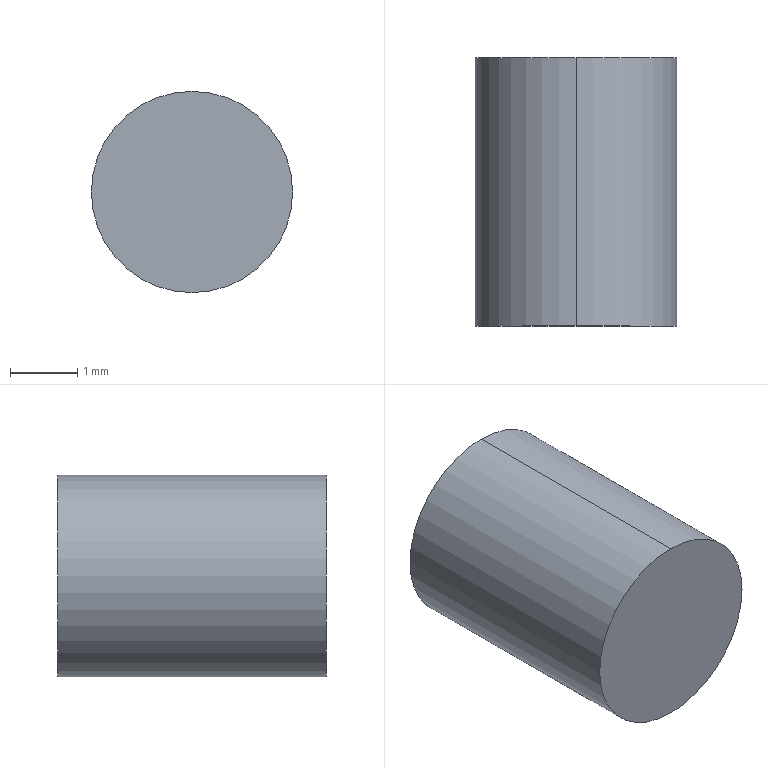Part | NX | features solid 2 | 1 solid | 4 faces | box 3 x 4 x 3 mm | volume 28.274 mm3 | plane 2 | cylinder 2 | commonest cylinder face diameters 3 x2
STEP:
#1=CARTESIAN_POINT('',(250.,-4.,-919.17));
#2=VERTEX_POINT('',#1);
#3=CARTESIAN_POINT('',(250.,-4.,-922.17));
#4=VERTEX_POINT('',#3);
#5=CARTESIAN_POINT('',(250.,-4.,-920.67));
#6=DIRECTION('',(0.,1.,0.));
#7=DIRECTION('',(0.,0.,1.));
#8=AXIS2_PLACEMENT_3D('',#5,#6,#7);
#9=CIRCLE('',#8,1.5);
#10=EDGE_CURVE('',#2,#4,#9,.T.);
#11=ORIENTED_EDGE('',*,*,#10,.F.);
#12=CARTESIAN_POINT('',(250.,-4.,-920.67));
#13=DIRECTION('',(0.,1.,0.));
#14=DIRECTION('',(0.,0.,-1.));
#15=AXIS2_PLACEMENT_3D('',#12,#13,#14);
#16=CIRCLE('',#15,1.5);
#17=EDGE_CURVE('',#4,#2,#16,.T.);
#18=ORIENTED_EDGE('',*,*,#17,.F.);
#19=EDGE_LOOP('',(#11,#18));
#20=FACE_BOUND('',#19,.T.);
#21=CARTESIAN_POINT('',(250.,-4.,-920.67));
#22=DIRECTION('',(0.,1.,0.));
#23=DIRECTION('',(0.,0.,1.));
#24=AXIS2_PLACEMENT_3D('',#21,#22,#23);
#25=PLANE('',#24);
#26=ADVANCED_FACE('',(#20),#25,.F.);
#27=CARTESIAN_POINT('',(250.,0.,-919.17));
#28=VERTEX_POINT('',#27);
#29=CARTESIAN_POINT('',(250.,-4.,-919.17));
#30=DIRECTION('',(0.,1.,0.));
#31=VECTOR('',#30,1000.);
#32=LINE('',#29,#31);
#33=EDGE_CURVE('',#2,#28,#32,.T.);
#34=ORIENTED_EDGE('',*,*,#33,.T.);
#35=CARTESIAN_POINT('',(250.,0.,-922.17));
#36=VERTEX_POINT('',#35);
#37=CARTESIAN_POINT('',(250.,0.,-920.67));
#38=DIRECTION('',(0.,-1.,0.));
#39=DIRECTION('',(0.,0.,1.));
#40=AXIS2_PLACEMENT_3D('',#37,#38,#39);
#41=CIRCLE('',#40,1.5);
#42=EDGE_CURVE('',#28,#36,#41,.T.);
#43=ORIENTED_EDGE('',*,*,#42,.T.);
#44=CARTESIAN_POINT('',(250.,-4.,-922.17));
#45=DIRECTION('',(0.,1.,0.));
#46=VECTOR('',#45,1000.);
#47=LINE('',#44,#46);
#48=EDGE_CURVE('',#36,#4,#47,.F.);
#49=ORIENTED_EDGE('',*,*,#48,.T.);
#50=ORIENTED_EDGE('',*,*,#17,.T.);
#51=EDGE_LOOP('',(#34,#43,#49,#50));
#52=FACE_BOUND('',#51,.T.);
#53=CARTESIAN_POINT('',(250.,-4.,-920.67));
#54=DIRECTION('',(0.,1.,0.));
#55=DIRECTION('',(0.,0.,1.));
#56=AXIS2_PLACEMENT_3D('',#53,#54,#55);
#57=CYLINDRICAL_SURFACE('',#56,1.5);
#58=ADVANCED_FACE('',(#52),#57,.T.);
#59=ORIENTED_EDGE('',*,*,#48,.F.);
#60=CARTESIAN_POINT('',(250.,0.,-920.67));
#61=DIRECTION('',(0.,-1.,0.));
#62=DIRECTION('',(0.,0.,-1.));
#63=AXIS2_PLACEMENT_3D('',#60,#61,#62);
#64=CIRCLE('',#63,1.5);
#65=EDGE_CURVE('',#36,#28,#64,.T.);
#66=ORIENTED_EDGE('',*,*,#65,.T.);
#67=ORIENTED_EDGE('',*,*,#33,.F.);
#68=ORIENTED_EDGE('',*,*,#10,.T.);
#69=EDGE_LOOP('',(#59,#66,#67,#68));
#70=FACE_BOUND('',#69,.T.);
#71=CARTESIAN_POINT('',(250.,-4.,-920.67));
#72=DIRECTION('',(0.,1.,0.));
#73=DIRECTION('',(0.,0.,1.));
#74=AXIS2_PLACEMENT_3D('',#71,#72,#73);
#75=CYLINDRICAL_SURFACE('',#74,1.5);
#76=ADVANCED_FACE('',(#70),#75,.T.);
#77=ORIENTED_EDGE('',*,*,#65,.F.);
#78=ORIENTED_EDGE('',*,*,#42,.F.);
#79=EDGE_LOOP('',(#77,#78));
#80=FACE_BOUND('',#79,.T.);
#81=CARTESIAN_POINT('',(250.,0.,-920.67));
#82=DIRECTION('',(0.,1.,0.));
#83=DIRECTION('',(0.,0.,1.));
#84=AXIS2_PLACEMENT_3D('',#81,#82,#83);
#85=PLANE('',#84);
#86=ADVANCED_FACE('',(#80),#85,.T.);
#87=CLOSED_SHELL('',(#26,#58,#76,#86));
#88=MANIFOLD_SOLID_BREP('',#87);
#89=(LENGTH_UNIT()NAMED_UNIT(*)SI_UNIT(.MILLI.,.METRE.));
#90=UNCERTAINTY_MEASURE_WITH_UNIT(LENGTH_MEASURE(0.00001),#89,'','');
#91=(NAMED_UNIT(*)PLANE_ANGLE_UNIT()SI_UNIT($,.RADIAN.));
#92=(NAMED_UNIT(*)SI_UNIT($,.STERADIAN.)SOLID_ANGLE_UNIT());
#93=(GEOMETRIC_REPRESENTATION_CONTEXT(3)GLOBAL_UNCERTAINTY_ASSIGNED_CONTEXT((#90))GLOBAL_UNIT_ASSIGNED_CONTEXT((#89,#91,#92))REPRESENTATION_CONTEXT('',''));
#94=ADVANCED_BREP_SHAPE_REPRESENTATION('',(#88),#93);